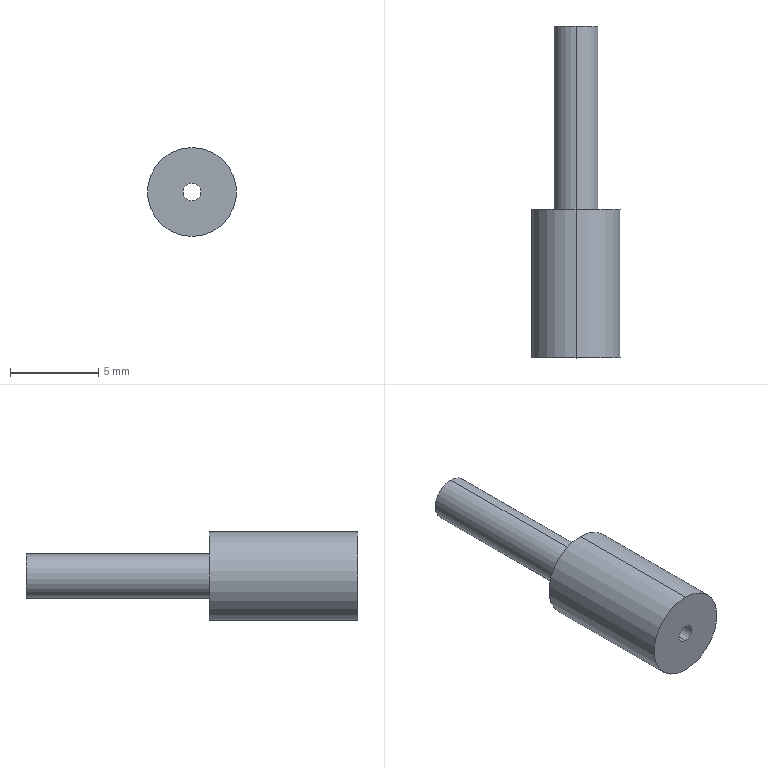Part | SolidWorks | features Revolution 1 | 1 solid | 9 faces | box 5.05 x 18.84 x 5.05 mm | volume 205.304 mm3 | cylinder 6 | plane 3 | commonest cylinder face diameters 1 x2 2.5 x2 5.05 x2
STEP:
#1=CARTESIAN_POINT('',(0.,8.44,1.25));
#2=VERTEX_POINT('',#1);
#3=CARTESIAN_POINT('',(0.,8.44,-1.25));
#4=VERTEX_POINT('',#3);
#5=CARTESIAN_POINT('',(0.,8.44,0.));
#6=DIRECTION('',(0.,1.,0.));
#7=DIRECTION('',(0.,0.,1.));
#8=AXIS2_PLACEMENT_3D('',#5,#6,#7);
#9=CIRCLE('',#8,1.25);
#10=EDGE_CURVE('',#2,#4,#9,.T.);
#11=ORIENTED_EDGE('',*,*,#10,.T.);
#12=CARTESIAN_POINT('',(0.,18.84,-1.25));
#13=VERTEX_POINT('',#12);
#14=CARTESIAN_POINT('',(0.,23.646,-1.25));
#15=DIRECTION('',(0.,1.,0.));
#16=VECTOR('',#15,1000.);
#17=LINE('',#14,#16);
#18=EDGE_CURVE('',#4,#13,#17,.T.);
#19=ORIENTED_EDGE('',*,*,#18,.T.);
#20=CARTESIAN_POINT('',(0.,18.84,1.25));
#21=VERTEX_POINT('',#20);
#22=CARTESIAN_POINT('',(0.,18.84,0.));
#23=DIRECTION('',(0.,1.,0.));
#24=DIRECTION('',(0.,0.,1.));
#25=AXIS2_PLACEMENT_3D('',#22,#23,#24);
#26=CIRCLE('',#25,1.25);
#27=EDGE_CURVE('',#21,#13,#26,.T.);
#28=ORIENTED_EDGE('',*,*,#27,.F.);
#29=CARTESIAN_POINT('',(0.,23.646,1.25));
#30=DIRECTION('',(0.,1.,0.));
#31=VECTOR('',#30,1000.);
#32=LINE('',#29,#31);
#33=EDGE_CURVE('',#2,#21,#32,.T.);
#34=ORIENTED_EDGE('',*,*,#33,.F.);
#35=EDGE_LOOP('',(#11,#19,#28,#34));
#36=FACE_OUTER_BOUND('',#35,.T.);
#37=CARTESIAN_POINT('',(0.,23.646,0.));
#38=DIRECTION('',(0.,1.,0.));
#39=DIRECTION('',(0.,0.,1.));
#40=AXIS2_PLACEMENT_3D('',#37,#38,#39);
#41=CYLINDRICAL_SURFACE('',#40,1.25);
#42=ADVANCED_FACE('',(#36),#41,.T.);
#43=CARTESIAN_POINT('',(0.,0.,2.525));
#44=VERTEX_POINT('',#43);
#45=CARTESIAN_POINT('',(0.,0.,-2.525));
#46=VERTEX_POINT('',#45);
#47=CARTESIAN_POINT('',(0.,0.,0.));
#48=DIRECTION('',(0.,1.,0.));
#49=DIRECTION('',(0.,0.,1.));
#50=AXIS2_PLACEMENT_3D('',#47,#48,#49);
#51=CIRCLE('',#50,2.525);
#52=EDGE_CURVE('',#44,#46,#51,.T.);
#53=ORIENTED_EDGE('',*,*,#52,.T.);
#54=CARTESIAN_POINT('',(0.,8.44,-2.525));
#55=VERTEX_POINT('',#54);
#56=CARTESIAN_POINT('',(0.,23.646,-2.525));
#57=DIRECTION('',(0.,1.,0.));
#58=VECTOR('',#57,1000.);
#59=LINE('',#56,#58);
#60=EDGE_CURVE('',#46,#55,#59,.T.);
#61=ORIENTED_EDGE('',*,*,#60,.T.);
#62=CARTESIAN_POINT('',(0.,8.44,2.525));
#63=VERTEX_POINT('',#62);
#64=CARTESIAN_POINT('',(0.,8.44,0.));
#65=DIRECTION('',(0.,1.,0.));
#66=DIRECTION('',(0.,0.,1.));
#67=AXIS2_PLACEMENT_3D('',#64,#65,#66);
#68=CIRCLE('',#67,2.525);
#69=EDGE_CURVE('',#63,#55,#68,.T.);
#70=ORIENTED_EDGE('',*,*,#69,.F.);
#71=CARTESIAN_POINT('',(0.,23.646,2.525));
#72=DIRECTION('',(0.,1.,0.));
#73=VECTOR('',#72,1000.);
#74=LINE('',#71,#73);
#75=EDGE_CURVE('',#44,#63,#74,.T.);
#76=ORIENTED_EDGE('',*,*,#75,.F.);
#77=EDGE_LOOP('',(#53,#61,#70,#76));
#78=FACE_OUTER_BOUND('',#77,.T.);
#79=CARTESIAN_POINT('',(0.,23.646,0.));
#80=DIRECTION('',(0.,1.,0.));
#81=DIRECTION('',(0.,0.,1.));
#82=AXIS2_PLACEMENT_3D('',#79,#80,#81);
#83=CYLINDRICAL_SURFACE('',#82,2.525);
#84=ADVANCED_FACE('',(#78),#83,.T.);
#85=CARTESIAN_POINT('',(0.,0.,-0.5));
#86=VERTEX_POINT('',#85);
#87=CARTESIAN_POINT('',(0.,0.,0.5));
#88=VERTEX_POINT('',#87);
#89=CARTESIAN_POINT('',(0.,0.,0.));
#90=DIRECTION('',(0.,1.,0.));
#91=DIRECTION('',(0.,0.,1.));
#92=AXIS2_PLACEMENT_3D('',#89,#90,#91);
#93=CIRCLE('',#92,0.5);
#94=EDGE_CURVE('',#86,#88,#93,.T.);
#95=ORIENTED_EDGE('',*,*,#94,.F.);
#96=CARTESIAN_POINT('',(0.,18.84,-0.5));
#97=VERTEX_POINT('',#96);
#98=CARTESIAN_POINT('',(0.,23.646,-0.5));
#99=DIRECTION('',(0.,1.,0.));
#100=VECTOR('',#99,1000.);
#101=LINE('',#98,#100);
#102=EDGE_CURVE('',#86,#97,#101,.T.);
#103=ORIENTED_EDGE('',*,*,#102,.T.);
#104=CARTESIAN_POINT('',(0.,18.84,0.5));
#105=VERTEX_POINT('',#104);
#106=CARTESIAN_POINT('',(0.,18.84,0.));
#107=DIRECTION('',(0.,1.,0.));
#108=DIRECTION('',(0.,0.,1.));
#109=AXIS2_PLACEMENT_3D('',#106,#107,#108);
#110=CIRCLE('',#109,0.5);
#111=EDGE_CURVE('',#97,#105,#110,.T.);
#112=ORIENTED_EDGE('',*,*,#111,.T.);
#113=CARTESIAN_POINT('',(0.,23.646,0.5));
#114=DIRECTION('',(0.,1.,0.));
#115=VECTOR('',#114,1000.);
#116=LINE('',#113,#115);
#117=EDGE_CURVE('',#88,#105,#116,.T.);
#118=ORIENTED_EDGE('',*,*,#117,.F.);
#119=EDGE_LOOP('',(#95,#103,#112,#118));
#120=FACE_OUTER_BOUND('',#119,.T.);
#121=CARTESIAN_POINT('',(0.,23.646,0.));
#122=DIRECTION('',(0.,1.,0.));
#123=DIRECTION('',(0.,0.,1.));
#124=AXIS2_PLACEMENT_3D('',#121,#122,#123);
#125=CYLINDRICAL_SURFACE('',#124,0.5);
#126=ADVANCED_FACE('',(#120),#125,.F.);
#127=ORIENTED_EDGE('',*,*,#27,.T.);
#128=CARTESIAN_POINT('',(0.,18.84,0.));
#129=DIRECTION('',(0.,1.,0.));
#130=DIRECTION('',(0.,0.,1.));
#131=AXIS2_PLACEMENT_3D('',#128,#129,#130);
#132=CIRCLE('',#131,1.25);
#133=EDGE_CURVE('',#13,#21,#132,.T.);
#134=ORIENTED_EDGE('',*,*,#133,.T.);
#135=EDGE_LOOP('',(#127,#134));
#136=FACE_OUTER_BOUND('',#135,.T.);
#137=CARTESIAN_POINT('',(0.,18.84,0.));
#138=DIRECTION('',(0.,1.,0.));
#139=DIRECTION('',(0.,0.,1.));
#140=AXIS2_PLACEMENT_3D('',#137,#138,#139);
#141=CIRCLE('',#140,0.5);
#142=EDGE_CURVE('',#105,#97,#141,.T.);
#143=ORIENTED_EDGE('',*,*,#142,.F.);
#144=ORIENTED_EDGE('',*,*,#111,.F.);
#145=EDGE_LOOP('',(#143,#144));
#146=FACE_BOUND('',#145,.T.);
#147=CARTESIAN_POINT('',(-1.25,18.84,0.));
#148=DIRECTION('',(0.,1.,0.));
#149=DIRECTION('',(0.,0.,1.));
#150=AXIS2_PLACEMENT_3D('',#147,#148,#149);
#151=PLANE('',#150);
#152=ADVANCED_FACE('',(#136,#146),#151,.T.);
#153=ORIENTED_EDGE('',*,*,#102,.F.);
#154=CARTESIAN_POINT('',(0.,0.,0.));
#155=DIRECTION('',(0.,1.,0.));
#156=DIRECTION('',(0.,0.,1.));
#157=AXIS2_PLACEMENT_3D('',#154,#155,#156);
#158=CIRCLE('',#157,0.5);
#159=EDGE_CURVE('',#88,#86,#158,.T.);
#160=ORIENTED_EDGE('',*,*,#159,.F.);
#161=ORIENTED_EDGE('',*,*,#117,.T.);
#162=ORIENTED_EDGE('',*,*,#142,.T.);
#163=EDGE_LOOP('',(#153,#160,#161,#162));
#164=FACE_OUTER_BOUND('',#163,.T.);
#165=CARTESIAN_POINT('',(0.,23.646,0.));
#166=DIRECTION('',(0.,1.,0.));
#167=DIRECTION('',(0.,0.,1.));
#168=AXIS2_PLACEMENT_3D('',#165,#166,#167);
#169=CYLINDRICAL_SURFACE('',#168,0.5);
#170=ADVANCED_FACE('',(#164),#169,.F.);
#171=ORIENTED_EDGE('',*,*,#159,.T.);
#172=ORIENTED_EDGE('',*,*,#94,.T.);
#173=EDGE_LOOP('',(#171,#172));
#174=FACE_BOUND('',#173,.T.);
#175=ORIENTED_EDGE('',*,*,#52,.F.);
#176=CARTESIAN_POINT('',(0.,0.,0.));
#177=DIRECTION('',(0.,1.,0.));
#178=DIRECTION('',(0.,0.,1.));
#179=AXIS2_PLACEMENT_3D('',#176,#177,#178);
#180=CIRCLE('',#179,2.525);
#181=EDGE_CURVE('',#46,#44,#180,.T.);
#182=ORIENTED_EDGE('',*,*,#181,.F.);
#183=EDGE_LOOP('',(#175,#182));
#184=FACE_OUTER_BOUND('',#183,.T.);
#185=CARTESIAN_POINT('',(-0.5,0.,0.));
#186=DIRECTION('',(0.,-1.,0.));
#187=DIRECTION('',(0.,0.,-1.));
#188=AXIS2_PLACEMENT_3D('',#185,#186,#187);
#189=PLANE('',#188);
#190=ADVANCED_FACE('',(#174,#184),#189,.T.);
#191=ORIENTED_EDGE('',*,*,#60,.F.);
#192=ORIENTED_EDGE('',*,*,#181,.T.);
#193=ORIENTED_EDGE('',*,*,#75,.T.);
#194=CARTESIAN_POINT('',(0.,8.44,0.));
#195=DIRECTION('',(0.,1.,0.));
#196=DIRECTION('',(0.,0.,1.));
#197=AXIS2_PLACEMENT_3D('',#194,#195,#196);
#198=CIRCLE('',#197,2.525);
#199=EDGE_CURVE('',#55,#63,#198,.T.);
#200=ORIENTED_EDGE('',*,*,#199,.F.);
#201=EDGE_LOOP('',(#191,#192,#193,#200));
#202=FACE_OUTER_BOUND('',#201,.T.);
#203=CARTESIAN_POINT('',(0.,23.646,0.));
#204=DIRECTION('',(0.,1.,0.));
#205=DIRECTION('',(0.,0.,1.));
#206=AXIS2_PLACEMENT_3D('',#203,#204,#205);
#207=CYLINDRICAL_SURFACE('',#206,2.525);
#208=ADVANCED_FACE('',(#202),#207,.T.);
#209=ORIENTED_EDGE('',*,*,#69,.T.);
#210=ORIENTED_EDGE('',*,*,#199,.T.);
#211=EDGE_LOOP('',(#209,#210));
#212=FACE_OUTER_BOUND('',#211,.T.);
#213=ORIENTED_EDGE('',*,*,#10,.F.);
#214=CARTESIAN_POINT('',(0.,8.44,0.));
#215=DIRECTION('',(0.,1.,0.));
#216=DIRECTION('',(0.,0.,1.));
#217=AXIS2_PLACEMENT_3D('',#214,#215,#216);
#218=CIRCLE('',#217,1.25);
#219=EDGE_CURVE('',#4,#2,#218,.T.);
#220=ORIENTED_EDGE('',*,*,#219,.F.);
#221=EDGE_LOOP('',(#213,#220));
#222=FACE_BOUND('',#221,.T.);
#223=CARTESIAN_POINT('',(-1.25,8.44,0.));
#224=DIRECTION('',(0.,1.,0.));
#225=DIRECTION('',(0.,0.,1.));
#226=AXIS2_PLACEMENT_3D('',#223,#224,#225);
#227=PLANE('',#226);
#228=ADVANCED_FACE('',(#212,#222),#227,.T.);
#229=ORIENTED_EDGE('',*,*,#18,.F.);
#230=ORIENTED_EDGE('',*,*,#219,.T.);
#231=ORIENTED_EDGE('',*,*,#33,.T.);
#232=ORIENTED_EDGE('',*,*,#133,.F.);
#233=EDGE_LOOP('',(#229,#230,#231,#232));
#234=FACE_OUTER_BOUND('',#233,.T.);
#235=CARTESIAN_POINT('',(0.,23.646,0.));
#236=DIRECTION('',(0.,1.,0.));
#237=DIRECTION('',(0.,0.,1.));
#238=AXIS2_PLACEMENT_3D('',#235,#236,#237);
#239=CYLINDRICAL_SURFACE('',#238,1.25);
#240=ADVANCED_FACE('',(#234),#239,.T.);
#241=CLOSED_SHELL('',(#42,#84,#126,#152,#170,#190,#208,#228,#240));
#242=MANIFOLD_SOLID_BREP('',#241);
#243=CARTESIAN_POINT('',(0.,0.,0.));
#244=DIRECTION('',(0.,0.,1.));
#245=DIRECTION('',(1.,0.,0.));
#246=AXIS2_PLACEMENT_3D('',#243,#244,#245);
#247=(LENGTH_UNIT()NAMED_UNIT(*)SI_UNIT(.MILLI.,.METRE.));
#248=UNCERTAINTY_MEASURE_WITH_UNIT(LENGTH_MEASURE(0.00001),#247,'','');
#249=(NAMED_UNIT(*)PLANE_ANGLE_UNIT()SI_UNIT($,.RADIAN.));
#250=(NAMED_UNIT(*)SI_UNIT($,.STERADIAN.)SOLID_ANGLE_UNIT());
#251=(GEOMETRIC_REPRESENTATION_CONTEXT(3)GLOBAL_UNCERTAINTY_ASSIGNED_CONTEXT((#248))GLOBAL_UNIT_ASSIGNED_CONTEXT((#247,#249,#250))REPRESENTATION_CONTEXT('',''));
#252=ADVANCED_BREP_SHAPE_REPRESENTATION('',(#242,#246),#251);